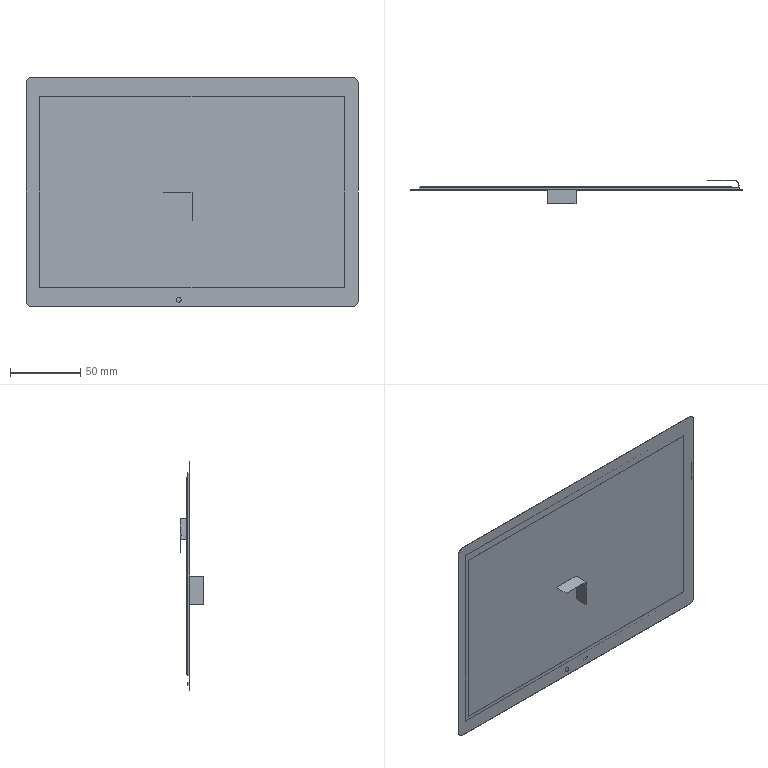Part | Creo | 1 solid | 58 faces | volume 51565 mm3 | plane 44 | cylinder 12 | other 2 | commonest cylinder face diameters 7.8 x4 2.2 x2 3.5 x2 6.9 x2 19.4 x1 20 x1